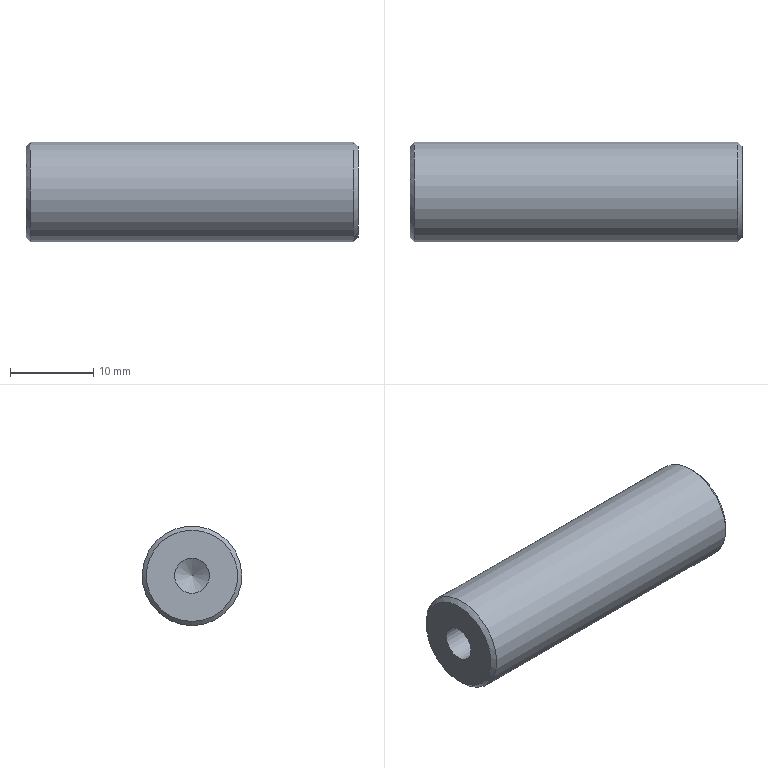Part | NX | 1 solid | 9 faces | box 40 x 12 x 12 mm | volume 4171 mm3 | cone 4 | cylinder 3 | plane 2 | commonest cylinder face diameters 4.2 x2 12 x1
STEP:
#1=CARTESIAN_POINT('',(19.5,0.,-6.));
#2=VERTEX_POINT('',#1);
#3=CARTESIAN_POINT('',(19.5,0.,0.));
#4=DIRECTION('',(1.,0.,0.));
#5=DIRECTION('',(0.,0.,-1.));
#6=AXIS2_PLACEMENT_3D('',#3,#4,#5);
#7=CIRCLE('',#6,6.);
#8=EDGE_CURVE('',#2,#2,#7,.F.);
#9=ORIENTED_EDGE('',*,*,#8,.T.);
#10=EDGE_LOOP('',(#9));
#11=FACE_BOUND('',#10,.T.);
#12=CARTESIAN_POINT('',(-19.5,0.,-6.));
#13=VERTEX_POINT('',#12);
#14=CARTESIAN_POINT('',(-19.5,0.,0.));
#15=DIRECTION('',(1.,0.,0.));
#16=DIRECTION('',(0.,0.,-1.));
#17=AXIS2_PLACEMENT_3D('',#14,#15,#16);
#18=CIRCLE('',#17,6.);
#19=EDGE_CURVE('',#13,#13,#18,.T.);
#20=ORIENTED_EDGE('',*,*,#19,.T.);
#21=EDGE_LOOP('',(#20));
#22=FACE_BOUND('',#21,.T.);
#23=CARTESIAN_POINT('',(20.,0.,0.));
#24=DIRECTION('',(-1.,0.,0.));
#25=DIRECTION('',(0.,0.,1.));
#26=AXIS2_PLACEMENT_3D('',#23,#24,#25);
#27=CYLINDRICAL_SURFACE('',#26,6.);
#28=ADVANCED_FACE('',(#11,#22),#27,.T.);
#29=CARTESIAN_POINT('',(20.,0.,-5.5));
#30=VERTEX_POINT('',#29);
#31=CARTESIAN_POINT('',(20.,0.,0.));
#32=DIRECTION('',(1.,0.,0.));
#33=DIRECTION('',(0.,0.,-1.));
#34=AXIS2_PLACEMENT_3D('',#31,#32,#33);
#35=CIRCLE('',#34,5.5);
#36=EDGE_CURVE('',#30,#30,#35,.T.);
#37=ORIENTED_EDGE('',*,*,#36,.T.);
#38=EDGE_LOOP('',(#37));
#39=FACE_BOUND('',#38,.T.);
#40=CARTESIAN_POINT('',(20.,0.,-2.1));
#41=VERTEX_POINT('',#40);
#42=CARTESIAN_POINT('',(20.,0.,0.));
#43=DIRECTION('',(1.,0.,0.));
#44=DIRECTION('',(0.,0.,-1.));
#45=AXIS2_PLACEMENT_3D('',#42,#43,#44);
#46=CIRCLE('',#45,2.1);
#47=EDGE_CURVE('',#41,#41,#46,.T.);
#48=ORIENTED_EDGE('',*,*,#47,.F.);
#49=EDGE_LOOP('',(#48));
#50=FACE_BOUND('',#49,.T.);
#51=CARTESIAN_POINT('',(20.,0.,0.));
#52=DIRECTION('',(1.,0.,0.));
#53=DIRECTION('',(0.,0.,-1.));
#54=AXIS2_PLACEMENT_3D('',#51,#52,#53);
#55=PLANE('',#54);
#56=ADVANCED_FACE('',(#39,#50),#55,.T.);
#57=CARTESIAN_POINT('',(-20.,0.,-5.5));
#58=VERTEX_POINT('',#57);
#59=CARTESIAN_POINT('',(-20.,0.,0.));
#60=DIRECTION('',(1.,0.,0.));
#61=DIRECTION('',(0.,0.,-1.));
#62=AXIS2_PLACEMENT_3D('',#59,#60,#61);
#63=CIRCLE('',#62,5.5);
#64=EDGE_CURVE('',#58,#58,#63,.F.);
#65=ORIENTED_EDGE('',*,*,#64,.T.);
#66=EDGE_LOOP('',(#65));
#67=FACE_BOUND('',#66,.T.);
#68=CARTESIAN_POINT('',(-20.,0.,2.1));
#69=VERTEX_POINT('',#68);
#70=CARTESIAN_POINT('',(-20.,0.,0.));
#71=DIRECTION('',(-1.,0.,0.));
#72=DIRECTION('',(0.,0.,1.));
#73=AXIS2_PLACEMENT_3D('',#70,#71,#72);
#74=CIRCLE('',#73,2.1);
#75=EDGE_CURVE('',#69,#69,#74,.T.);
#76=ORIENTED_EDGE('',*,*,#75,.F.);
#77=EDGE_LOOP('',(#76));
#78=FACE_BOUND('',#77,.T.);
#79=CARTESIAN_POINT('',(-20.,0.,0.));
#80=DIRECTION('',(1.,0.,0.));
#81=DIRECTION('',(0.,0.,-1.));
#82=AXIS2_PLACEMENT_3D('',#79,#80,#81);
#83=PLANE('',#82);
#84=ADVANCED_FACE('',(#67,#78),#83,.F.);
#85=CARTESIAN_POINT('',(-6.738,0.,0.));
#86=VERTEX_POINT('',#85);
#87=VERTEX_LOOP('',#86);
#88=FACE_BOUND('',#87,.T.);
#89=CARTESIAN_POINT('',(-8.,0.,2.1));
#90=VERTEX_POINT('',#89);
#91=CARTESIAN_POINT('',(-8.,0.,0.));
#92=DIRECTION('',(-1.,0.,0.));
#93=DIRECTION('',(0.,0.,1.));
#94=AXIS2_PLACEMENT_3D('',#91,#92,#93);
#95=CIRCLE('',#94,2.1);
#96=EDGE_CURVE('',#90,#90,#95,.T.);
#97=ORIENTED_EDGE('',*,*,#96,.T.);
#98=EDGE_LOOP('',(#97));
#99=FACE_BOUND('',#98,.T.);
#100=CARTESIAN_POINT('',(-8.,0.,0.));
#101=DIRECTION('',(-1.,0.,0.));
#102=DIRECTION('',(0.,0.,1.));
#103=AXIS2_PLACEMENT_3D('',#100,#101,#102);
#104=CONICAL_SURFACE('',#103,2.1,1.03);
#105=ADVANCED_FACE('',(#88,#99),#104,.F.);
#106=ORIENTED_EDGE('',*,*,#96,.F.);
#107=EDGE_LOOP('',(#106));
#108=FACE_BOUND('',#107,.T.);
#109=ORIENTED_EDGE('',*,*,#75,.T.);
#110=EDGE_LOOP('',(#109));
#111=FACE_BOUND('',#110,.T.);
#112=CARTESIAN_POINT('',(-20.,0.,0.));
#113=DIRECTION('',(-1.,0.,0.));
#114=DIRECTION('',(0.,0.,1.));
#115=AXIS2_PLACEMENT_3D('',#112,#113,#114);
#116=CYLINDRICAL_SURFACE('',#115,2.1);
#117=ADVANCED_FACE('',(#108,#111),#116,.F.);
#118=CARTESIAN_POINT('',(6.738,0.,0.));
#119=VERTEX_POINT('',#118);
#120=VERTEX_LOOP('',#119);
#121=FACE_BOUND('',#120,.T.);
#122=CARTESIAN_POINT('',(8.,0.,-2.1));
#123=VERTEX_POINT('',#122);
#124=CARTESIAN_POINT('',(8.,0.,0.));
#125=DIRECTION('',(1.,0.,0.));
#126=DIRECTION('',(0.,0.,-1.));
#127=AXIS2_PLACEMENT_3D('',#124,#125,#126);
#128=CIRCLE('',#127,2.1);
#129=EDGE_CURVE('',#123,#123,#128,.T.);
#130=ORIENTED_EDGE('',*,*,#129,.T.);
#131=EDGE_LOOP('',(#130));
#132=FACE_BOUND('',#131,.T.);
#133=CARTESIAN_POINT('',(8.,0.,0.));
#134=DIRECTION('',(1.,0.,0.));
#135=DIRECTION('',(0.,0.,-1.));
#136=AXIS2_PLACEMENT_3D('',#133,#134,#135);
#137=CONICAL_SURFACE('',#136,2.1,1.03);
#138=ADVANCED_FACE('',(#121,#132),#137,.F.);
#139=ORIENTED_EDGE('',*,*,#129,.F.);
#140=EDGE_LOOP('',(#139));
#141=FACE_BOUND('',#140,.T.);
#142=ORIENTED_EDGE('',*,*,#47,.T.);
#143=EDGE_LOOP('',(#142));
#144=FACE_BOUND('',#143,.T.);
#145=CARTESIAN_POINT('',(20.,0.,0.));
#146=DIRECTION('',(1.,0.,0.));
#147=DIRECTION('',(0.,0.,-1.));
#148=AXIS2_PLACEMENT_3D('',#145,#146,#147);
#149=CYLINDRICAL_SURFACE('',#148,2.1);
#150=ADVANCED_FACE('',(#141,#144),#149,.F.);
#151=ORIENTED_EDGE('',*,*,#8,.F.);
#152=EDGE_LOOP('',(#151));
#153=FACE_BOUND('',#152,.T.);
#154=ORIENTED_EDGE('',*,*,#36,.F.);
#155=EDGE_LOOP('',(#154));
#156=FACE_BOUND('',#155,.T.);
#157=CARTESIAN_POINT('',(20.,0.,0.));
#158=DIRECTION('',(-1.,0.,0.));
#159=DIRECTION('',(0.,0.,1.));
#160=AXIS2_PLACEMENT_3D('',#157,#158,#159);
#161=CONICAL_SURFACE('',#160,5.5,0.7854);
#162=ADVANCED_FACE('',(#153,#156),#161,.T.);
#163=ORIENTED_EDGE('',*,*,#64,.F.);
#164=EDGE_LOOP('',(#163));
#165=FACE_BOUND('',#164,.T.);
#166=ORIENTED_EDGE('',*,*,#19,.F.);
#167=EDGE_LOOP('',(#166));
#168=FACE_BOUND('',#167,.T.);
#169=CARTESIAN_POINT('',(-19.5,0.,0.));
#170=DIRECTION('',(1.,0.,0.));
#171=DIRECTION('',(0.,0.,-1.));
#172=AXIS2_PLACEMENT_3D('',#169,#170,#171);
#173=CONICAL_SURFACE('',#172,6.,0.7854);
#174=ADVANCED_FACE('',(#165,#168),#173,.T.);
#175=CLOSED_SHELL('',(#28,#56,#84,#105,#117,#138,#150,#162,#174));
#176=MANIFOLD_SOLID_BREP('',#175);
#177=(LENGTH_UNIT()NAMED_UNIT(*)SI_UNIT(.MILLI.,.METRE.));
#178=UNCERTAINTY_MEASURE_WITH_UNIT(LENGTH_MEASURE(0.00001),#177,'','');
#179=(NAMED_UNIT(*)PLANE_ANGLE_UNIT()SI_UNIT($,.RADIAN.));
#180=(NAMED_UNIT(*)SI_UNIT($,.STERADIAN.)SOLID_ANGLE_UNIT());
#181=(GEOMETRIC_REPRESENTATION_CONTEXT(3)GLOBAL_UNCERTAINTY_ASSIGNED_CONTEXT((#178))GLOBAL_UNIT_ASSIGNED_CONTEXT((#177,#179,#180))REPRESENTATION_CONTEXT('',''));
#182=ADVANCED_BREP_SHAPE_REPRESENTATION('',(#176),#181);